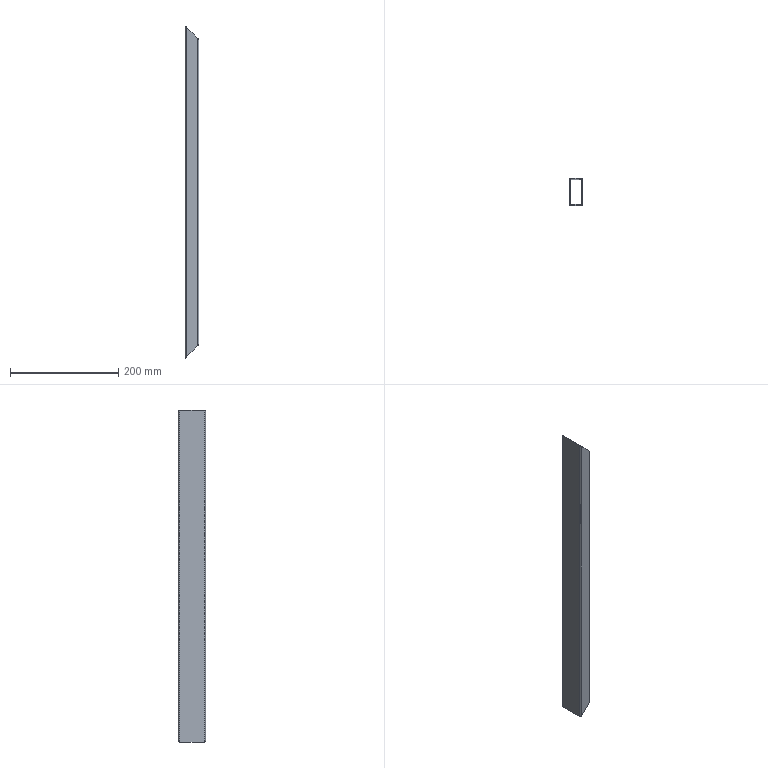Part | STEP file | 7100519 | 1 solid | 18 faces | box 25 x 50 x 613 mm | volume 124358 mm3 | plane 10 | cylinder 8 | commonest cylinder face diameters 2 x4 5 x4